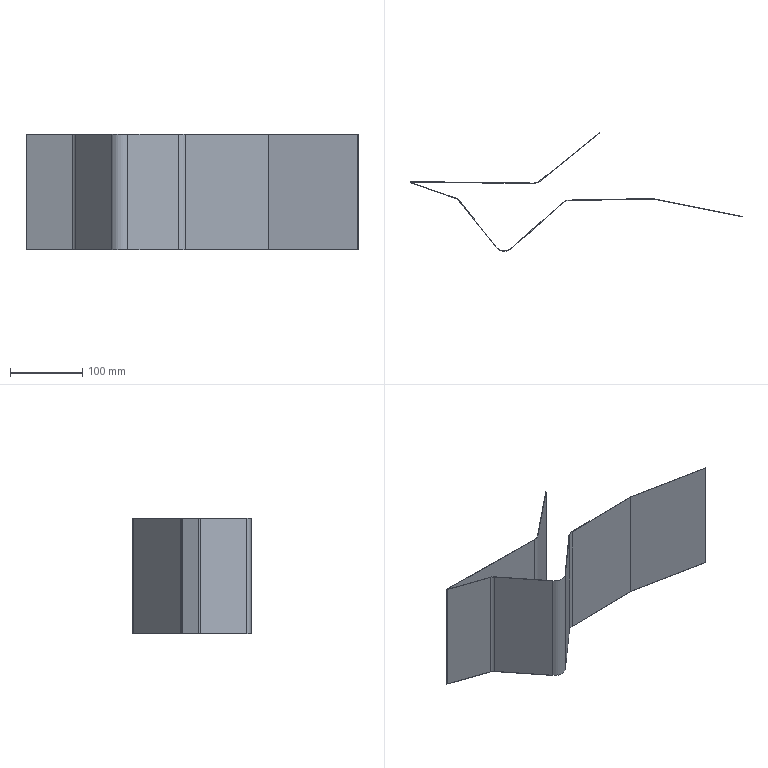Part | STEP file | Layout^ | 1 solid | 30 faces | box 459.008 x 163.495 x 160 mm | volume 64878 mm3 | plane 20 | cylinder 10 | commonest cylinder face diameters 30 x4 29 x2 31 x2 19 x1 20 x1
STEP:
#1=CARTESIAN_POINT('',(-164.589,156.602,25.));
#2=VERTEX_POINT('',#1);
#3=CARTESIAN_POINT('',(-41.59,132.165,25.));
#4=VERTEX_POINT('',#3);
#5=CARTESIAN_POINT('',(-164.642,156.612,25.));
#6=DIRECTION('',(0.9808,-0.1949,0.));
#7=VECTOR('',#6,1000.);
#8=LINE('',#5,#7);
#9=EDGE_CURVE('',#2,#4,#8,.T.);
#10=ORIENTED_EDGE('',*,*,#9,.T.);
#11=CARTESIAN_POINT('',(-41.59,132.165,185.));
#12=VERTEX_POINT('',#11);
#13=CARTESIAN_POINT('',(-41.59,132.165,185.));
#14=DIRECTION('',(0.,0.,-1.));
#15=VECTOR('',#14,1000.);
#16=LINE('',#13,#15);
#17=EDGE_CURVE('',#12,#4,#16,.T.);
#18=ORIENTED_EDGE('',*,*,#17,.F.);
#19=CARTESIAN_POINT('',(-164.589,156.602,185.));
#20=VERTEX_POINT('',#19);
#21=CARTESIAN_POINT('',(-164.642,156.612,185.));
#22=DIRECTION('',(0.9808,-0.1949,0.));
#23=VECTOR('',#22,1000.);
#24=LINE('',#21,#23);
#25=EDGE_CURVE('',#20,#12,#24,.T.);
#26=ORIENTED_EDGE('',*,*,#25,.F.);
#27=CARTESIAN_POINT('',(-164.589,156.602,185.));
#28=DIRECTION('',(0.,0.,-1.));
#29=VECTOR('',#28,1000.);
#30=LINE('',#27,#29);
#31=EDGE_CURVE('',#20,#2,#30,.T.);
#32=ORIENTED_EDGE('',*,*,#31,.T.);
#33=EDGE_LOOP('',(#10,#18,#26,#32));
#34=FACE_OUTER_BOUND('',#33,.T.);
#35=CARTESIAN_POINT('',(-164.642,156.612,185.));
#36=DIRECTION('',(0.1949,0.9808,0.));
#37=DIRECTION('',(-0.9808,0.1949,0.));
#38=AXIS2_PLACEMENT_3D('',#35,#36,#37);
#39=PLANE('',#38);
#40=ADVANCED_FACE('',(#34),#39,.F.);
#41=CARTESIAN_POINT('',(-41.492,132.655,25.));
#42=VERTEX_POINT('',#41);
#43=CARTESIAN_POINT('',(-41.492,132.655,25.));
#44=DIRECTION('',(-0.1949,-0.9808,0.));
#45=VECTOR('',#44,1000.);
#46=LINE('',#43,#45);
#47=EDGE_CURVE('',#42,#4,#46,.T.);
#48=ORIENTED_EDGE('',*,*,#47,.F.);
#49=CARTESIAN_POINT('',(-41.492,132.655,185.));
#50=VERTEX_POINT('',#49);
#51=CARTESIAN_POINT('',(-41.492,132.655,185.));
#52=DIRECTION('',(0.,0.,-1.));
#53=VECTOR('',#52,1000.);
#54=LINE('',#51,#53);
#55=EDGE_CURVE('',#50,#42,#54,.T.);
#56=ORIENTED_EDGE('',*,*,#55,.F.);
#57=CARTESIAN_POINT('',(-41.492,132.655,185.));
#58=DIRECTION('',(-0.1949,-0.9808,0.));
#59=VECTOR('',#58,1000.);
#60=LINE('',#57,#59);
#61=EDGE_CURVE('',#50,#12,#60,.T.);
#62=ORIENTED_EDGE('',*,*,#61,.T.);
#63=ORIENTED_EDGE('',*,*,#17,.T.);
#64=EDGE_LOOP('',(#48,#56,#62,#63));
#65=FACE_OUTER_BOUND('',#64,.T.);
#66=CARTESIAN_POINT('',(-41.492,132.655,185.));
#67=DIRECTION('',(0.9808,-0.1949,0.));
#68=DIRECTION('',(0.1949,0.9808,0.));
#69=AXIS2_PLACEMENT_3D('',#66,#67,#68);
#70=PLANE('',#69);
#71=ADVANCED_FACE('',(#65),#70,.T.);
#72=CARTESIAN_POINT('',(-164.544,157.103,25.));
#73=VERTEX_POINT('',#72);
#74=CARTESIAN_POINT('',(-164.544,157.103,25.));
#75=DIRECTION('',(0.9808,-0.1949,0.));
#76=VECTOR('',#75,1000.);
#77=LINE('',#74,#76);
#78=EDGE_CURVE('',#73,#42,#77,.T.);
#79=ORIENTED_EDGE('',*,*,#78,.F.);
#80=CARTESIAN_POINT('',(-164.544,157.103,185.));
#81=VERTEX_POINT('',#80);
#82=CARTESIAN_POINT('',(-164.544,157.103,185.));
#83=DIRECTION('',(0.,0.,-1.));
#84=VECTOR('',#83,1000.);
#85=LINE('',#82,#84);
#86=EDGE_CURVE('',#81,#73,#85,.T.);
#87=ORIENTED_EDGE('',*,*,#86,.F.);
#88=CARTESIAN_POINT('',(-164.544,157.103,185.));
#89=DIRECTION('',(0.9808,-0.1949,0.));
#90=VECTOR('',#89,1000.);
#91=LINE('',#88,#90);
#92=EDGE_CURVE('',#81,#50,#91,.T.);
#93=ORIENTED_EDGE('',*,*,#92,.T.);
#94=ORIENTED_EDGE('',*,*,#55,.T.);
#95=EDGE_LOOP('',(#79,#87,#93,#94));
#96=FACE_OUTER_BOUND('',#95,.T.);
#97=CARTESIAN_POINT('',(-164.544,157.103,185.));
#98=DIRECTION('',(0.1949,0.9808,0.));
#99=DIRECTION('',(-0.9808,0.1949,0.));
#100=AXIS2_PLACEMENT_3D('',#97,#98,#99);
#101=PLANE('',#100);
#102=ADVANCED_FACE('',(#96),#101,.T.);
#103=CARTESIAN_POINT('',(-280.273,154.998,25.));
#104=VERTEX_POINT('',#103);
#105=CARTESIAN_POINT('',(-280.273,154.998,25.));
#106=DIRECTION('',(0.9998,0.01819,0.));
#107=VECTOR('',#106,1000.);
#108=LINE('',#105,#107);
#109=EDGE_CURVE('',#104,#73,#108,.T.);
#110=ORIENTED_EDGE('',*,*,#109,.F.);
#111=CARTESIAN_POINT('',(-280.273,154.998,185.));
#112=VERTEX_POINT('',#111);
#113=CARTESIAN_POINT('',(-280.273,154.998,185.));
#114=DIRECTION('',(0.,0.,-1.));
#115=VECTOR('',#114,1000.);
#116=LINE('',#113,#115);
#117=EDGE_CURVE('',#112,#104,#116,.T.);
#118=ORIENTED_EDGE('',*,*,#117,.F.);
#119=CARTESIAN_POINT('',(-280.273,154.998,185.));
#120=DIRECTION('',(0.9998,0.01819,0.));
#121=VECTOR('',#120,1000.);
#122=LINE('',#119,#121);
#123=EDGE_CURVE('',#112,#81,#122,.T.);
#124=ORIENTED_EDGE('',*,*,#123,.T.);
#125=ORIENTED_EDGE('',*,*,#86,.T.);
#126=EDGE_LOOP('',(#110,#118,#124,#125));
#127=FACE_OUTER_BOUND('',#126,.T.);
#128=CARTESIAN_POINT('',(-280.273,154.998,185.));
#129=DIRECTION('',(-0.01819,0.9998,0.));
#130=DIRECTION('',(-0.9998,-0.01819,0.));
#131=AXIS2_PLACEMENT_3D('',#128,#129,#130);
#132=PLANE('',#131);
#133=ADVANCED_FACE('',(#127),#132,.T.);
#134=CARTESIAN_POINT('',(-289.978,151.2,25.));
#135=VERTEX_POINT('',#134);
#136=CARTESIAN_POINT('',(-280.,140.,25.));
#137=DIRECTION('',(0.,0.,-1.));
#138=DIRECTION('',(-1.,0.,0.));
#139=AXIS2_PLACEMENT_3D('',#136,#137,#138);
#140=CIRCLE('',#139,15.);
#141=EDGE_CURVE('',#135,#104,#140,.T.);
#142=ORIENTED_EDGE('',*,*,#141,.F.);
#143=CARTESIAN_POINT('',(-289.978,151.2,185.));
#144=VERTEX_POINT('',#143);
#145=CARTESIAN_POINT('',(-289.978,151.2,185.));
#146=DIRECTION('',(0.,0.,-1.));
#147=VECTOR('',#146,1000.);
#148=LINE('',#145,#147);
#149=EDGE_CURVE('',#144,#135,#148,.T.);
#150=ORIENTED_EDGE('',*,*,#149,.F.);
#151=CARTESIAN_POINT('',(-280.,140.,185.));
#152=DIRECTION('',(0.,0.,-1.));
#153=DIRECTION('',(-1.,0.,0.));
#154=AXIS2_PLACEMENT_3D('',#151,#152,#153);
#155=CIRCLE('',#154,15.);
#156=EDGE_CURVE('',#144,#112,#155,.T.);
#157=ORIENTED_EDGE('',*,*,#156,.T.);
#158=ORIENTED_EDGE('',*,*,#117,.T.);
#159=EDGE_LOOP('',(#142,#150,#157,#158));
#160=FACE_OUTER_BOUND('',#159,.T.);
#161=CARTESIAN_POINT('',(-280.,140.,185.));
#162=DIRECTION('',(0.,0.,-1.));
#163=DIRECTION('',(-1.,0.,0.));
#164=AXIS2_PLACEMENT_3D('',#161,#162,#163);
#165=CYLINDRICAL_SURFACE('',#164,15.);
#166=ADVANCED_FACE('',(#160),#165,.T.);
#167=CARTESIAN_POINT('',(-360.022,88.8,25.));
#168=VERTEX_POINT('',#167);
#169=CARTESIAN_POINT('',(-360.022,88.8,25.));
#170=DIRECTION('',(0.7467,0.6652,0.));
#171=VECTOR('',#170,1000.);
#172=LINE('',#169,#171);
#173=EDGE_CURVE('',#168,#135,#172,.T.);
#174=ORIENTED_EDGE('',*,*,#173,.F.);
#175=CARTESIAN_POINT('',(-360.022,88.8,185.));
#176=VERTEX_POINT('',#175);
#177=CARTESIAN_POINT('',(-360.022,88.8,185.));
#178=DIRECTION('',(0.,0.,-1.));
#179=VECTOR('',#178,1000.);
#180=LINE('',#177,#179);
#181=EDGE_CURVE('',#176,#168,#180,.T.);
#182=ORIENTED_EDGE('',*,*,#181,.F.);
#183=CARTESIAN_POINT('',(-360.022,88.8,185.));
#184=DIRECTION('',(0.7467,0.6652,0.));
#185=VECTOR('',#184,1000.);
#186=LINE('',#183,#185);
#187=EDGE_CURVE('',#176,#144,#186,.T.);
#188=ORIENTED_EDGE('',*,*,#187,.T.);
#189=ORIENTED_EDGE('',*,*,#149,.T.);
#190=EDGE_LOOP('',(#174,#182,#188,#189));
#191=FACE_OUTER_BOUND('',#190,.T.);
#192=CARTESIAN_POINT('',(-360.022,88.8,185.));
#193=DIRECTION('',(-0.6652,0.7467,0.));
#194=DIRECTION('',(-0.7467,-0.6652,0.));
#195=AXIS2_PLACEMENT_3D('',#192,#193,#194);
#196=PLANE('',#195);
#197=ADVANCED_FACE('',(#191),#196,.T.);
#198=CARTESIAN_POINT('',(-381.75,90.676,25.));
#199=VERTEX_POINT('',#198);
#200=CARTESIAN_POINT('',(-370.,100.,25.));
#201=DIRECTION('',(0.,0.,1.));
#202=DIRECTION('',(1.,0.,0.));
#203=AXIS2_PLACEMENT_3D('',#200,#201,#202);
#204=CIRCLE('',#203,15.);
#205=EDGE_CURVE('',#199,#168,#204,.T.);
#206=ORIENTED_EDGE('',*,*,#205,.F.);
#207=CARTESIAN_POINT('',(-381.75,90.676,185.));
#208=VERTEX_POINT('',#207);
#209=CARTESIAN_POINT('',(-381.75,90.676,185.));
#210=DIRECTION('',(0.,0.,-1.));
#211=VECTOR('',#210,1000.);
#212=LINE('',#209,#211);
#213=EDGE_CURVE('',#208,#199,#212,.T.);
#214=ORIENTED_EDGE('',*,*,#213,.F.);
#215=CARTESIAN_POINT('',(-370.,100.,185.));
#216=DIRECTION('',(0.,0.,1.));
#217=DIRECTION('',(1.,0.,0.));
#218=AXIS2_PLACEMENT_3D('',#215,#216,#217);
#219=CIRCLE('',#218,15.);
#220=EDGE_CURVE('',#208,#176,#219,.T.);
#221=ORIENTED_EDGE('',*,*,#220,.T.);
#222=ORIENTED_EDGE('',*,*,#181,.T.);
#223=EDGE_LOOP('',(#206,#214,#221,#222));
#224=FACE_OUTER_BOUND('',#223,.T.);
#225=CARTESIAN_POINT('',(-370.,100.,185.));
#226=DIRECTION('',(0.,0.,-1.));
#227=DIRECTION('',(-1.,0.,0.));
#228=AXIS2_PLACEMENT_3D('',#225,#226,#227);
#229=CYLINDRICAL_SURFACE('',#228,15.);
#230=ADVANCED_FACE('',(#224),#229,.F.);
#231=CARTESIAN_POINT('',(-432.166,154.216,25.));
#232=VERTEX_POINT('',#231);
#233=CARTESIAN_POINT('',(-432.166,154.216,25.));
#234=DIRECTION('',(0.6216,-0.7834,0.));
#235=VECTOR('',#234,1000.);
#236=LINE('',#233,#235);
#237=EDGE_CURVE('',#232,#199,#236,.T.);
#238=ORIENTED_EDGE('',*,*,#237,.F.);
#239=CARTESIAN_POINT('',(-432.166,154.216,185.));
#240=VERTEX_POINT('',#239);
#241=CARTESIAN_POINT('',(-432.166,154.216,185.));
#242=DIRECTION('',(0.,0.,-1.));
#243=VECTOR('',#242,1000.);
#244=LINE('',#241,#243);
#245=EDGE_CURVE('',#240,#232,#244,.T.);
#246=ORIENTED_EDGE('',*,*,#245,.F.);
#247=CARTESIAN_POINT('',(-432.166,154.216,185.));
#248=DIRECTION('',(0.6216,-0.7834,0.));
#249=VECTOR('',#248,1000.);
#250=LINE('',#247,#249);
#251=EDGE_CURVE('',#240,#208,#250,.T.);
#252=ORIENTED_EDGE('',*,*,#251,.T.);
#253=ORIENTED_EDGE('',*,*,#213,.T.);
#254=EDGE_LOOP('',(#238,#246,#252,#253));
#255=FACE_OUTER_BOUND('',#254,.T.);
#256=CARTESIAN_POINT('',(-432.166,154.216,185.));
#257=DIRECTION('',(0.7834,0.6216,0.));
#258=DIRECTION('',(-0.6216,0.7834,0.));
#259=AXIS2_PLACEMENT_3D('',#256,#257,#258);
#260=PLANE('',#259);
#261=ADVANCED_FACE('',(#255),#260,.T.);
#262=CARTESIAN_POINT('',(-436.696,157.438,25.));
#263=VERTEX_POINT('',#262);
#264=CARTESIAN_POINT('',(-440.,148.,25.));
#265=DIRECTION('',(0.,0.,-1.));
#266=DIRECTION('',(1.,0.,0.));
#267=AXIS2_PLACEMENT_3D('',#264,#265,#266);
#268=CIRCLE('',#267,10.);
#269=EDGE_CURVE('',#263,#232,#268,.T.);
#270=ORIENTED_EDGE('',*,*,#269,.F.);
#271=CARTESIAN_POINT('',(-436.696,157.438,185.));
#272=VERTEX_POINT('',#271);
#273=CARTESIAN_POINT('',(-436.696,157.438,185.));
#274=DIRECTION('',(0.,0.,-1.));
#275=VECTOR('',#274,1000.);
#276=LINE('',#273,#275);
#277=EDGE_CURVE('',#272,#263,#276,.T.);
#278=ORIENTED_EDGE('',*,*,#277,.F.);
#279=CARTESIAN_POINT('',(-440.,148.,185.));
#280=DIRECTION('',(0.,0.,-1.));
#281=DIRECTION('',(1.,0.,0.));
#282=AXIS2_PLACEMENT_3D('',#279,#280,#281);
#283=CIRCLE('',#282,10.);
#284=EDGE_CURVE('',#272,#240,#283,.T.);
#285=ORIENTED_EDGE('',*,*,#284,.T.);
#286=ORIENTED_EDGE('',*,*,#245,.T.);
#287=EDGE_LOOP('',(#270,#278,#285,#286));
#288=FACE_OUTER_BOUND('',#287,.T.);
#289=CARTESIAN_POINT('',(-440.,148.,185.));
#290=DIRECTION('',(0.,0.,-1.));
#291=DIRECTION('',(-1.,0.,0.));
#292=AXIS2_PLACEMENT_3D('',#289,#290,#291);
#293=CYLINDRICAL_SURFACE('',#292,10.);
#294=ADVANCED_FACE('',(#288),#293,.T.);
#295=CARTESIAN_POINT('',(-500.,179.6,25.));
#296=VERTEX_POINT('',#295);
#297=CARTESIAN_POINT('',(-500.,179.6,25.));
#298=DIRECTION('',(0.9438,-0.3304,0.));
#299=VECTOR('',#298,1000.);
#300=LINE('',#297,#299);
#301=EDGE_CURVE('',#296,#263,#300,.T.);
#302=ORIENTED_EDGE('',*,*,#301,.F.);
#303=CARTESIAN_POINT('',(-500.,179.6,185.));
#304=VERTEX_POINT('',#303);
#305=CARTESIAN_POINT('',(-500.,179.6,185.));
#306=DIRECTION('',(0.,0.,-1.));
#307=VECTOR('',#306,1000.);
#308=LINE('',#305,#307);
#309=EDGE_CURVE('',#304,#296,#308,.T.);
#310=ORIENTED_EDGE('',*,*,#309,.F.);
#311=CARTESIAN_POINT('',(-500.,179.6,185.));
#312=DIRECTION('',(0.9438,-0.3304,0.));
#313=VECTOR('',#312,1000.);
#314=LINE('',#311,#313);
#315=EDGE_CURVE('',#304,#272,#314,.T.);
#316=ORIENTED_EDGE('',*,*,#315,.T.);
#317=ORIENTED_EDGE('',*,*,#277,.T.);
#318=EDGE_LOOP('',(#302,#310,#316,#317));
#319=FACE_OUTER_BOUND('',#318,.T.);
#320=CARTESIAN_POINT('',(-500.,179.6,185.));
#321=DIRECTION('',(0.3304,0.9438,0.));
#322=DIRECTION('',(-0.9438,0.3304,0.));
#323=AXIS2_PLACEMENT_3D('',#320,#321,#322);
#324=PLANE('',#323);
#325=ADVANCED_FACE('',(#319),#324,.T.);
#326=CARTESIAN_POINT('',(-500.,180.,25.));
#327=VERTEX_POINT('',#326);
#328=CARTESIAN_POINT('',(-500.,180.,25.));
#329=DIRECTION('',(0.,-1.,0.));
#330=VECTOR('',#329,1000.);
#331=LINE('',#328,#330);
#332=EDGE_CURVE('',#327,#296,#331,.T.);
#333=ORIENTED_EDGE('',*,*,#332,.F.);
#334=CARTESIAN_POINT('',(-500.,180.,185.));
#335=VERTEX_POINT('',#334);
#336=CARTESIAN_POINT('',(-500.,180.,185.));
#337=DIRECTION('',(0.,0.,-1.));
#338=VECTOR('',#337,1000.);
#339=LINE('',#336,#338);
#340=EDGE_CURVE('',#335,#327,#339,.T.);
#341=ORIENTED_EDGE('',*,*,#340,.F.);
#342=CARTESIAN_POINT('',(-500.,180.,185.));
#343=DIRECTION('',(0.,-1.,0.));
#344=VECTOR('',#343,1000.);
#345=LINE('',#342,#344);
#346=EDGE_CURVE('',#335,#304,#345,.T.);
#347=ORIENTED_EDGE('',*,*,#346,.T.);
#348=ORIENTED_EDGE('',*,*,#309,.T.);
#349=EDGE_LOOP('',(#333,#341,#347,#348));
#350=FACE_OUTER_BOUND('',#349,.T.);
#351=CARTESIAN_POINT('',(-500.,180.,185.));
#352=DIRECTION('',(1.,0.,0.));
#353=DIRECTION('',(0.,0.,-1.));
#354=AXIS2_PLACEMENT_3D('',#351,#352,#353);
#355=PLANE('',#354);
#356=ADVANCED_FACE('',(#350),#355,.T.);
#357=CARTESIAN_POINT('',(-330.177,178.001,25.));
#358=VERTEX_POINT('',#357);
#359=CARTESIAN_POINT('',(-330.177,178.001,25.));
#360=DIRECTION('',(-0.9999,0.01177,0.));
#361=VECTOR('',#360,1000.);
#362=LINE('',#359,#361);
#363=EDGE_CURVE('',#358,#327,#362,.T.);
#364=ORIENTED_EDGE('',*,*,#363,.F.);
#365=CARTESIAN_POINT('',(-330.177,178.001,185.));
#366=VERTEX_POINT('',#365);
#367=CARTESIAN_POINT('',(-330.177,178.001,185.));
#368=DIRECTION('',(0.,0.,-1.));
#369=VECTOR('',#368,1000.);
#370=LINE('',#367,#369);
#371=EDGE_CURVE('',#366,#358,#370,.T.);
#372=ORIENTED_EDGE('',*,*,#371,.F.);
#373=CARTESIAN_POINT('',(-330.177,178.001,185.));
#374=DIRECTION('',(-0.9999,0.01177,0.));
#375=VECTOR('',#374,1000.);
#376=LINE('',#373,#375);
#377=EDGE_CURVE('',#366,#335,#376,.T.);
#378=ORIENTED_EDGE('',*,*,#377,.T.);
#379=ORIENTED_EDGE('',*,*,#340,.T.);
#380=EDGE_LOOP('',(#364,#372,#378,#379));
#381=FACE_OUTER_BOUND('',#380,.T.);
#382=CARTESIAN_POINT('',(-330.177,178.001,185.));
#383=DIRECTION('',(-0.01177,-0.9999,0.));
#384=DIRECTION('',(0.9999,-0.01177,0.));
#385=AXIS2_PLACEMENT_3D('',#382,#383,#384);
#386=PLANE('',#385);
#387=ADVANCED_FACE('',(#381),#386,.T.);
#388=CARTESIAN_POINT('',(-320.593,181.316,25.));
#389=VERTEX_POINT('',#388);
#390=CARTESIAN_POINT('',(-330.,193.,25.));
#391=DIRECTION('',(0.,0.,-1.));
#392=DIRECTION('',(-1.,0.,0.));
#393=AXIS2_PLACEMENT_3D('',#390,#391,#392);
#394=CIRCLE('',#393,15.);
#395=EDGE_CURVE('',#389,#358,#394,.T.);
#396=ORIENTED_EDGE('',*,*,#395,.F.);
#397=CARTESIAN_POINT('',(-320.593,181.316,185.));
#398=VERTEX_POINT('',#397);
#399=CARTESIAN_POINT('',(-320.593,181.316,185.));
#400=DIRECTION('',(0.,0.,-1.));
#401=VECTOR('',#400,1000.);
#402=LINE('',#399,#401);
#403=EDGE_CURVE('',#398,#389,#402,.T.);
#404=ORIENTED_EDGE('',*,*,#403,.F.);
#405=CARTESIAN_POINT('',(-330.,193.,185.));
#406=DIRECTION('',(0.,0.,-1.));
#407=DIRECTION('',(-1.,0.,0.));
#408=AXIS2_PLACEMENT_3D('',#405,#406,#407);
#409=CIRCLE('',#408,15.);
#410=EDGE_CURVE('',#398,#366,#409,.T.);
#411=ORIENTED_EDGE('',*,*,#410,.T.);
#412=ORIENTED_EDGE('',*,*,#371,.T.);
#413=EDGE_LOOP('',(#396,#404,#411,#412));
#414=FACE_OUTER_BOUND('',#413,.T.);
#415=CARTESIAN_POINT('',(-330.,193.,185.));
#416=DIRECTION('',(0.,0.,-1.));
#417=DIRECTION('',(-1.,0.,0.));
#418=AXIS2_PLACEMENT_3D('',#415,#416,#417);
#419=CYLINDRICAL_SURFACE('',#418,15.);
#420=ADVANCED_FACE('',(#414),#419,.T.);
#421=CARTESIAN_POINT('',(-239.407,246.684,25.));
#422=VERTEX_POINT('',#421);
#423=CARTESIAN_POINT('',(-239.407,246.684,25.));
#424=DIRECTION('',(-0.7789,-0.6271,0.));
#425=VECTOR('',#424,1000.);
#426=LINE('',#423,#425);
#427=EDGE_CURVE('',#422,#389,#426,.T.);
#428=ORIENTED_EDGE('',*,*,#427,.F.);
#429=CARTESIAN_POINT('',(-239.407,246.684,185.));
#430=VERTEX_POINT('',#429);
#431=CARTESIAN_POINT('',(-239.407,246.684,185.));
#432=DIRECTION('',(0.,0.,-1.));
#433=VECTOR('',#432,1000.);
#434=LINE('',#431,#433);
#435=EDGE_CURVE('',#430,#422,#434,.T.);
#436=ORIENTED_EDGE('',*,*,#435,.F.);
#437=CARTESIAN_POINT('',(-239.407,246.684,185.));
#438=DIRECTION('',(-0.7789,-0.6271,0.));
#439=VECTOR('',#438,1000.);
#440=LINE('',#437,#439);
#441=EDGE_CURVE('',#430,#398,#440,.T.);
#442=ORIENTED_EDGE('',*,*,#441,.T.);
#443=ORIENTED_EDGE('',*,*,#403,.T.);
#444=EDGE_LOOP('',(#428,#436,#442,#443));
#445=FACE_OUTER_BOUND('',#444,.T.);
#446=CARTESIAN_POINT('',(-239.407,246.684,185.));
#447=DIRECTION('',(0.6271,-0.7789,0.));
#448=DIRECTION('',(0.7789,0.6271,0.));
#449=AXIS2_PLACEMENT_3D('',#446,#447,#448);
#450=PLANE('',#449);
#451=ADVANCED_FACE('',(#445),#450,.T.);
#452=CARTESIAN_POINT('',(-238.176,247.576,25.));
#453=VERTEX_POINT('',#452);
#454=CARTESIAN_POINT('',(-230.,235.,25.));
#455=DIRECTION('',(0.,0.,1.));
#456=DIRECTION('',(-1.,0.,0.));
#457=AXIS2_PLACEMENT_3D('',#454,#455,#456);
#458=CIRCLE('',#457,15.);
#459=EDGE_CURVE('',#453,#422,#458,.T.);
#460=ORIENTED_EDGE('',*,*,#459,.F.);
#461=CARTESIAN_POINT('',(-238.176,247.576,185.));
#462=VERTEX_POINT('',#461);
#463=CARTESIAN_POINT('',(-238.176,247.576,185.));
#464=DIRECTION('',(0.,0.,-1.));
#465=VECTOR('',#464,1000.);
#466=LINE('',#463,#465);
#467=EDGE_CURVE('',#462,#453,#466,.T.);
#468=ORIENTED_EDGE('',*,*,#467,.F.);
#469=CARTESIAN_POINT('',(-230.,235.,185.));
#470=DIRECTION('',(0.,0.,1.));
#471=DIRECTION('',(-1.,0.,0.));
#472=AXIS2_PLACEMENT_3D('',#469,#470,#471);
#473=CIRCLE('',#472,15.);
#474=EDGE_CURVE('',#462,#430,#473,.T.);
#475=ORIENTED_EDGE('',*,*,#474,.T.);
#476=ORIENTED_EDGE('',*,*,#435,.T.);
#477=EDGE_LOOP('',(#460,#468,#475,#476));
#478=FACE_OUTER_BOUND('',#477,.T.);
#479=CARTESIAN_POINT('',(-230.,235.,185.));
#480=DIRECTION('',(0.,0.,-1.));
#481=DIRECTION('',(-1.,0.,0.));
#482=AXIS2_PLACEMENT_3D('',#479,#480,#481);
#483=CYLINDRICAL_SURFACE('',#482,15.);
#484=ADVANCED_FACE('',(#478),#483,.F.);
#485=CARTESIAN_POINT('',(-238.448,247.995,25.));
#486=VERTEX_POINT('',#485);
#487=CARTESIAN_POINT('',(-238.448,247.995,25.));
#488=DIRECTION('',(0.545,-0.8384,0.));
#489=VECTOR('',#488,1000.);
#490=LINE('',#487,#489);
#491=EDGE_CURVE('',#486,#453,#490,.T.);
#492=ORIENTED_EDGE('',*,*,#491,.F.);
#493=CARTESIAN_POINT('',(-238.448,247.995,185.));
#494=VERTEX_POINT('',#493);
#495=CARTESIAN_POINT('',(-238.448,247.995,185.));
#496=DIRECTION('',(0.,0.,-1.));
#497=VECTOR('',#496,1000.);
#498=LINE('',#495,#497);
#499=EDGE_CURVE('',#494,#486,#498,.T.);
#500=ORIENTED_EDGE('',*,*,#499,.F.);
#501=CARTESIAN_POINT('',(-238.448,247.995,185.));
#502=DIRECTION('',(0.545,-0.8384,0.));
#503=VECTOR('',#502,1000.);
#504=LINE('',#501,#503);
#505=EDGE_CURVE('',#494,#462,#504,.T.);
#506=ORIENTED_EDGE('',*,*,#505,.T.);
#507=ORIENTED_EDGE('',*,*,#467,.T.);
#508=EDGE_LOOP('',(#492,#500,#506,#507));
#509=FACE_OUTER_BOUND('',#508,.T.);
#510=CARTESIAN_POINT('',(-238.448,247.995,185.));
#511=DIRECTION('',(0.8384,0.545,0.));
#512=DIRECTION('',(-0.545,0.8384,0.));
#513=AXIS2_PLACEMENT_3D('',#510,#511,#512);
#514=PLANE('',#513);
#515=ADVANCED_FACE('',(#509),#514,.T.);
#516=CARTESIAN_POINT('',(-239.721,247.073,25.));
#517=VERTEX_POINT('',#516);
#518=CARTESIAN_POINT('',(-230.,235.,25.));
#519=DIRECTION('',(0.,0.,1.));
#520=DIRECTION('',(1.,0.,0.));
#521=AXIS2_PLACEMENT_3D('',#518,#519,#520);
#522=CIRCLE('',#521,15.5);
#523=EDGE_CURVE('',#486,#517,#522,.T.);
#524=ORIENTED_EDGE('',*,*,#523,.T.);
#525=CARTESIAN_POINT('',(-239.721,247.073,185.));
#526=VERTEX_POINT('',#525);
#527=CARTESIAN_POINT('',(-239.721,247.073,185.));
#528=DIRECTION('',(0.,0.,-1.));
#529=VECTOR('',#528,1000.);
#530=LINE('',#527,#529);
#531=EDGE_CURVE('',#526,#517,#530,.T.);
#532=ORIENTED_EDGE('',*,*,#531,.F.);
#533=CARTESIAN_POINT('',(-230.,235.,185.));
#534=DIRECTION('',(0.,0.,1.));
#535=DIRECTION('',(1.,0.,0.));
#536=AXIS2_PLACEMENT_3D('',#533,#534,#535);
#537=CIRCLE('',#536,15.5);
#538=EDGE_CURVE('',#494,#526,#537,.T.);
#539=ORIENTED_EDGE('',*,*,#538,.F.);
#540=ORIENTED_EDGE('',*,*,#499,.T.);
#541=EDGE_LOOP('',(#524,#532,#539,#540));
#542=FACE_OUTER_BOUND('',#541,.T.);
#543=CARTESIAN_POINT('',(-230.,235.,185.));
#544=DIRECTION('',(0.,0.,-1.));
#545=DIRECTION('',(-1.,0.,0.));
#546=AXIS2_PLACEMENT_3D('',#543,#544,#545);
#547=CYLINDRICAL_SURFACE('',#546,15.5);
#548=ADVANCED_FACE('',(#542),#547,.T.);
#549=CARTESIAN_POINT('',(-320.906,181.706,25.));
#550=VERTEX_POINT('',#549);
#551=CARTESIAN_POINT('',(-239.721,247.073,25.));
#552=DIRECTION('',(-0.7789,-0.6271,0.));
#553=VECTOR('',#552,1000.);
#554=LINE('',#551,#553);
#555=EDGE_CURVE('',#517,#550,#554,.T.);
#556=ORIENTED_EDGE('',*,*,#555,.T.);
#557=CARTESIAN_POINT('',(-320.906,181.706,185.));
#558=VERTEX_POINT('',#557);
#559=CARTESIAN_POINT('',(-320.906,181.706,185.));
#560=DIRECTION('',(0.,0.,-1.));
#561=VECTOR('',#560,1000.);
#562=LINE('',#559,#561);
#563=EDGE_CURVE('',#558,#550,#562,.T.);
#564=ORIENTED_EDGE('',*,*,#563,.F.);
#565=CARTESIAN_POINT('',(-239.721,247.073,185.));
#566=DIRECTION('',(-0.7789,-0.6271,0.));
#567=VECTOR('',#566,1000.);
#568=LINE('',#565,#567);
#569=EDGE_CURVE('',#526,#558,#568,.T.);
#570=ORIENTED_EDGE('',*,*,#569,.F.);
#571=ORIENTED_EDGE('',*,*,#531,.T.);
#572=EDGE_LOOP('',(#556,#564,#570,#571));
#573=FACE_OUTER_BOUND('',#572,.T.);
#574=CARTESIAN_POINT('',(-239.721,247.073,185.));
#575=DIRECTION('',(0.6271,-0.7789,0.));
#576=DIRECTION('',(0.7789,0.6271,0.));
#577=AXIS2_PLACEMENT_3D('',#574,#575,#576);
#578=PLANE('',#577);
#579=ADVANCED_FACE('',(#573),#578,.F.);
#580=CARTESIAN_POINT('',(-330.171,178.501,25.));
#581=VERTEX_POINT('',#580);
#582=CARTESIAN_POINT('',(-330.,193.,25.));
#583=DIRECTION('',(0.,0.,-1.));
#584=DIRECTION('',(1.,0.,0.));
#585=AXIS2_PLACEMENT_3D('',#582,#583,#584);
#586=CIRCLE('',#585,14.5);
#587=EDGE_CURVE('',#550,#581,#586,.T.);
#588=ORIENTED_EDGE('',*,*,#587,.T.);
#589=CARTESIAN_POINT('',(-330.171,178.501,185.));
#590=VERTEX_POINT('',#589);
#591=CARTESIAN_POINT('',(-330.171,178.501,185.));
#592=DIRECTION('',(0.,0.,-1.));
#593=VECTOR('',#592,1000.);
#594=LINE('',#591,#593);
#595=EDGE_CURVE('',#590,#581,#594,.T.);
#596=ORIENTED_EDGE('',*,*,#595,.F.);
#597=CARTESIAN_POINT('',(-330.,193.,185.));
#598=DIRECTION('',(0.,0.,-1.));
#599=DIRECTION('',(1.,0.,0.));
#600=AXIS2_PLACEMENT_3D('',#597,#598,#599);
#601=CIRCLE('',#600,14.5);
#602=EDGE_CURVE('',#558,#590,#601,.T.);
#603=ORIENTED_EDGE('',*,*,#602,.F.);
#604=ORIENTED_EDGE('',*,*,#563,.T.);
#605=EDGE_LOOP('',(#588,#596,#603,#604));
#606=FACE_OUTER_BOUND('',#605,.T.);
#607=CARTESIAN_POINT('',(-330.,193.,185.));
#608=DIRECTION('',(0.,0.,-1.));
#609=DIRECTION('',(-1.,0.,0.));
#610=AXIS2_PLACEMENT_3D('',#607,#608,#609);
#611=CYLINDRICAL_SURFACE('',#610,14.5);
#612=ADVANCED_FACE('',(#606),#611,.F.);
#613=CARTESIAN_POINT('',(-500.5,180.506,25.));
#614=VERTEX_POINT('',#613);
#615=CARTESIAN_POINT('',(-330.171,178.501,25.));
#616=DIRECTION('',(-0.9999,0.01177,0.));
#617=VECTOR('',#616,1000.);
#618=LINE('',#615,#617);
#619=EDGE_CURVE('',#581,#614,#618,.T.);
#620=ORIENTED_EDGE('',*,*,#619,.T.);
#621=CARTESIAN_POINT('',(-500.5,180.506,185.));
#622=VERTEX_POINT('',#621);
#623=CARTESIAN_POINT('',(-500.5,180.506,185.));
#624=DIRECTION('',(0.,0.,-1.));
#625=VECTOR('',#624,1000.);
#626=LINE('',#623,#625);
#627=EDGE_CURVE('',#622,#614,#626,.T.);
#628=ORIENTED_EDGE('',*,*,#627,.F.);
#629=CARTESIAN_POINT('',(-330.171,178.501,185.));
#630=DIRECTION('',(-0.9999,0.01177,0.));
#631=VECTOR('',#630,1000.);
#632=LINE('',#629,#631);
#633=EDGE_CURVE('',#590,#622,#632,.T.);
#634=ORIENTED_EDGE('',*,*,#633,.F.);
#635=ORIENTED_EDGE('',*,*,#595,.T.);
#636=EDGE_LOOP('',(#620,#628,#634,#635));
#637=FACE_OUTER_BOUND('',#636,.T.);
#638=CARTESIAN_POINT('',(-330.171,178.501,185.));
#639=DIRECTION('',(-0.01177,-0.9999,0.));
#640=DIRECTION('',(0.9999,-0.01177,0.));
#641=AXIS2_PLACEMENT_3D('',#638,#639,#640);
#642=PLANE('',#641);
#643=ADVANCED_FACE('',(#637),#642,.F.);
#644=CARTESIAN_POINT('',(-500.5,179.245,25.));
#645=VERTEX_POINT('',#644);
#646=CARTESIAN_POINT('',(-500.5,180.,25.));
#647=DIRECTION('',(0.,-1.,0.));
#648=VECTOR('',#647,1000.);
#649=LINE('',#646,#648);
#650=EDGE_CURVE('',#614,#645,#649,.T.);
#651=ORIENTED_EDGE('',*,*,#650,.T.);
#652=CARTESIAN_POINT('',(-500.5,179.245,185.));
#653=VERTEX_POINT('',#652);
#654=CARTESIAN_POINT('',(-500.5,179.245,185.));
#655=DIRECTION('',(0.,0.,-1.));
#656=VECTOR('',#655,1000.);
#657=LINE('',#654,#656);
#658=EDGE_CURVE('',#653,#645,#657,.T.);
#659=ORIENTED_EDGE('',*,*,#658,.F.);
#660=CARTESIAN_POINT('',(-500.5,180.,185.));
#661=DIRECTION('',(0.,-1.,0.));
#662=VECTOR('',#661,1000.);
#663=LINE('',#660,#662);
#664=EDGE_CURVE('',#622,#653,#663,.T.);
#665=ORIENTED_EDGE('',*,*,#664,.F.);
#666=ORIENTED_EDGE('',*,*,#627,.T.);
#667=EDGE_LOOP('',(#651,#659,#665,#666));
#668=FACE_OUTER_BOUND('',#667,.T.);
#669=CARTESIAN_POINT('',(-500.5,180.,185.));
#670=DIRECTION('',(1.,0.,0.));
#671=DIRECTION('',(0.,0.,-1.));
#672=AXIS2_PLACEMENT_3D('',#669,#670,#671);
#673=PLANE('',#672);
#674=ADVANCED_FACE('',(#668),#673,.F.);
#675=CARTESIAN_POINT('',(-436.861,156.966,25.));
#676=VERTEX_POINT('',#675);
#677=CARTESIAN_POINT('',(-500.165,179.128,25.));
#678=DIRECTION('',(0.9438,-0.3304,0.));
#679=VECTOR('',#678,1000.);
#680=LINE('',#677,#679);
#681=EDGE_CURVE('',#645,#676,#680,.T.);
#682=ORIENTED_EDGE('',*,*,#681,.T.);
#683=CARTESIAN_POINT('',(-436.861,156.966,185.));
#684=VERTEX_POINT('',#683);
#685=CARTESIAN_POINT('',(-436.861,156.966,185.));
#686=DIRECTION('',(0.,0.,-1.));
#687=VECTOR('',#686,1000.);
#688=LINE('',#685,#687);
#689=EDGE_CURVE('',#684,#676,#688,.T.);
#690=ORIENTED_EDGE('',*,*,#689,.F.);
#691=CARTESIAN_POINT('',(-500.165,179.128,185.));
#692=DIRECTION('',(0.9438,-0.3304,0.));
#693=VECTOR('',#692,1000.);
#694=LINE('',#691,#693);
#695=EDGE_CURVE('',#653,#684,#694,.T.);
#696=ORIENTED_EDGE('',*,*,#695,.F.);
#697=ORIENTED_EDGE('',*,*,#658,.T.);
#698=EDGE_LOOP('',(#682,#690,#696,#697));
#699=FACE_OUTER_BOUND('',#698,.T.);
#700=CARTESIAN_POINT('',(-500.165,179.128,185.));
#701=DIRECTION('',(0.3304,0.9438,0.));
#702=DIRECTION('',(-0.9438,0.3304,0.));
#703=AXIS2_PLACEMENT_3D('',#700,#701,#702);
#704=PLANE('',#703);
#705=ADVANCED_FACE('',(#699),#704,.F.);
#706=CARTESIAN_POINT('',(-432.558,153.905,25.));
#707=VERTEX_POINT('',#706);
#708=CARTESIAN_POINT('',(-440.,148.,25.));
#709=DIRECTION('',(0.,0.,-1.));
#710=DIRECTION('',(1.,0.,0.));
#711=AXIS2_PLACEMENT_3D('',#708,#709,#710);
#712=CIRCLE('',#711,9.5);
#713=EDGE_CURVE('',#676,#707,#712,.T.);
#714=ORIENTED_EDGE('',*,*,#713,.T.);
#715=CARTESIAN_POINT('',(-432.558,153.905,185.));
#716=VERTEX_POINT('',#715);
#717=CARTESIAN_POINT('',(-432.558,153.905,185.));
#718=DIRECTION('',(0.,0.,-1.));
#719=VECTOR('',#718,1000.);
#720=LINE('',#717,#719);
#721=EDGE_CURVE('',#716,#707,#720,.T.);
#722=ORIENTED_EDGE('',*,*,#721,.F.);
#723=CARTESIAN_POINT('',(-440.,148.,185.));
#724=DIRECTION('',(0.,0.,-1.));
#725=DIRECTION('',(1.,0.,0.));
#726=AXIS2_PLACEMENT_3D('',#723,#724,#725);
#727=CIRCLE('',#726,9.5);
#728=EDGE_CURVE('',#684,#716,#727,.T.);
#729=ORIENTED_EDGE('',*,*,#728,.F.);
#730=ORIENTED_EDGE('',*,*,#689,.T.);
#731=EDGE_LOOP('',(#714,#722,#729,#730));
#732=FACE_OUTER_BOUND('',#731,.T.);
#733=CARTESIAN_POINT('',(-440.,148.,185.));
#734=DIRECTION('',(0.,0.,-1.));
#735=DIRECTION('',(-1.,0.,0.));
#736=AXIS2_PLACEMENT_3D('',#733,#734,#735);
#737=CYLINDRICAL_SURFACE('',#736,9.5);
#738=ADVANCED_FACE('',(#732),#737,.F.);
#739=CARTESIAN_POINT('',(-382.142,90.366,25.));
#740=VERTEX_POINT('',#739);
#741=CARTESIAN_POINT('',(-432.558,153.905,25.));
#742=DIRECTION('',(0.6216,-0.7834,0.));
#743=VECTOR('',#742,1000.);
#744=LINE('',#741,#743);
#745=EDGE_CURVE('',#707,#740,#744,.T.);
#746=ORIENTED_EDGE('',*,*,#745,.T.);
#747=CARTESIAN_POINT('',(-382.142,90.366,185.));
#748=VERTEX_POINT('',#747);
#749=CARTESIAN_POINT('',(-382.142,90.366,185.));
#750=DIRECTION('',(0.,0.,-1.));
#751=VECTOR('',#750,1000.);
#752=LINE('',#749,#751);
#753=EDGE_CURVE('',#748,#740,#752,.T.);
#754=ORIENTED_EDGE('',*,*,#753,.F.);
#755=CARTESIAN_POINT('',(-432.558,153.905,185.));
#756=DIRECTION('',(0.6216,-0.7834,0.));
#757=VECTOR('',#756,1000.);
#758=LINE('',#755,#757);
#759=EDGE_CURVE('',#716,#748,#758,.T.);
#760=ORIENTED_EDGE('',*,*,#759,.F.);
#761=ORIENTED_EDGE('',*,*,#721,.T.);
#762=EDGE_LOOP('',(#746,#754,#760,#761));
#763=FACE_OUTER_BOUND('',#762,.T.);
#764=CARTESIAN_POINT('',(-432.558,153.905,185.));
#765=DIRECTION('',(0.7834,0.6216,0.));
#766=DIRECTION('',(-0.6216,0.7834,0.));
#767=AXIS2_PLACEMENT_3D('',#764,#765,#766);
#768=PLANE('',#767);
#769=ADVANCED_FACE('',(#763),#768,.F.);
#770=CARTESIAN_POINT('',(-359.69,88.427,25.));
#771=VERTEX_POINT('',#770);
#772=CARTESIAN_POINT('',(-370.,100.,25.));
#773=DIRECTION('',(0.,0.,1.));
#774=DIRECTION('',(1.,0.,0.));
#775=AXIS2_PLACEMENT_3D('',#772,#773,#774);
#776=CIRCLE('',#775,15.5);
#777=EDGE_CURVE('',#740,#771,#776,.T.);
#778=ORIENTED_EDGE('',*,*,#777,.T.);
#779=CARTESIAN_POINT('',(-359.69,88.427,185.));
#780=VERTEX_POINT('',#779);
#781=CARTESIAN_POINT('',(-359.69,88.427,185.));
#782=DIRECTION('',(0.,0.,-1.));
#783=VECTOR('',#782,1000.);
#784=LINE('',#781,#783);
#785=EDGE_CURVE('',#780,#771,#784,.T.);
#786=ORIENTED_EDGE('',*,*,#785,.F.);
#787=CARTESIAN_POINT('',(-370.,100.,185.));
#788=DIRECTION('',(0.,0.,1.));
#789=DIRECTION('',(1.,0.,0.));
#790=AXIS2_PLACEMENT_3D('',#787,#788,#789);
#791=CIRCLE('',#790,15.5);
#792=EDGE_CURVE('',#748,#780,#791,.T.);
#793=ORIENTED_EDGE('',*,*,#792,.F.);
#794=ORIENTED_EDGE('',*,*,#753,.T.);
#795=EDGE_LOOP('',(#778,#786,#793,#794));
#796=FACE_OUTER_BOUND('',#795,.T.);
#797=CARTESIAN_POINT('',(-370.,100.,185.));
#798=DIRECTION('',(0.,0.,-1.));
#799=DIRECTION('',(-1.,0.,0.));
#800=AXIS2_PLACEMENT_3D('',#797,#798,#799);
#801=CYLINDRICAL_SURFACE('',#800,15.5);
#802=ADVANCED_FACE('',(#796),#801,.T.);
#803=CARTESIAN_POINT('',(-289.645,150.827,25.));
#804=VERTEX_POINT('',#803);
#805=CARTESIAN_POINT('',(-359.69,88.427,25.));
#806=DIRECTION('',(0.7467,0.6652,0.));
#807=VECTOR('',#806,1000.);
#808=LINE('',#805,#807);
#809=EDGE_CURVE('',#771,#804,#808,.T.);
#810=ORIENTED_EDGE('',*,*,#809,.T.);
#811=CARTESIAN_POINT('',(-289.645,150.827,185.));
#812=VERTEX_POINT('',#811);
#813=CARTESIAN_POINT('',(-289.645,150.827,185.));
#814=DIRECTION('',(0.,0.,-1.));
#815=VECTOR('',#814,1000.);
#816=LINE('',#813,#815);
#817=EDGE_CURVE('',#812,#804,#816,.T.);
#818=ORIENTED_EDGE('',*,*,#817,.F.);
#819=CARTESIAN_POINT('',(-359.69,88.427,185.));
#820=DIRECTION('',(0.7467,0.6652,0.));
#821=VECTOR('',#820,1000.);
#822=LINE('',#819,#821);
#823=EDGE_CURVE('',#780,#812,#822,.T.);
#824=ORIENTED_EDGE('',*,*,#823,.F.);
#825=ORIENTED_EDGE('',*,*,#785,.T.);
#826=EDGE_LOOP('',(#810,#818,#824,#825));
#827=FACE_OUTER_BOUND('',#826,.T.);
#828=CARTESIAN_POINT('',(-359.69,88.427,185.));
#829=DIRECTION('',(-0.6652,0.7467,0.));
#830=DIRECTION('',(-0.7467,-0.6652,0.));
#831=AXIS2_PLACEMENT_3D('',#828,#829,#830);
#832=PLANE('',#831);
#833=ADVANCED_FACE('',(#827),#832,.F.);
#834=CARTESIAN_POINT('',(-280.264,154.498,25.));
#835=VERTEX_POINT('',#834);
#836=CARTESIAN_POINT('',(-280.,140.,25.));
#837=DIRECTION('',(0.,0.,-1.));
#838=DIRECTION('',(1.,0.,0.));
#839=AXIS2_PLACEMENT_3D('',#836,#837,#838);
#840=CIRCLE('',#839,14.5);
#841=EDGE_CURVE('',#804,#835,#840,.T.);
#842=ORIENTED_EDGE('',*,*,#841,.T.);
#843=CARTESIAN_POINT('',(-280.264,154.498,185.));
#844=VERTEX_POINT('',#843);
#845=CARTESIAN_POINT('',(-280.264,154.498,185.));
#846=DIRECTION('',(0.,0.,-1.));
#847=VECTOR('',#846,1000.);
#848=LINE('',#845,#847);
#849=EDGE_CURVE('',#844,#835,#848,.T.);
#850=ORIENTED_EDGE('',*,*,#849,.F.);
#851=CARTESIAN_POINT('',(-280.,140.,185.));
#852=DIRECTION('',(0.,0.,-1.));
#853=DIRECTION('',(1.,0.,0.));
#854=AXIS2_PLACEMENT_3D('',#851,#852,#853);
#855=CIRCLE('',#854,14.5);
#856=EDGE_CURVE('',#812,#844,#855,.T.);
#857=ORIENTED_EDGE('',*,*,#856,.F.);
#858=ORIENTED_EDGE('',*,*,#817,.T.);
#859=EDGE_LOOP('',(#842,#850,#857,#858));
#860=FACE_OUTER_BOUND('',#859,.T.);
#861=CARTESIAN_POINT('',(-280.,140.,185.));
#862=DIRECTION('',(0.,0.,-1.));
#863=DIRECTION('',(-1.,0.,0.));
#864=AXIS2_PLACEMENT_3D('',#861,#862,#863);
#865=CYLINDRICAL_SURFACE('',#864,14.5);
#866=ADVANCED_FACE('',(#860),#865,.F.);
#867=CARTESIAN_POINT('',(-280.264,154.498,25.));
#868=DIRECTION('',(0.9998,0.01819,0.));
#869=VECTOR('',#868,1000.);
#870=LINE('',#867,#869);
#871=EDGE_CURVE('',#835,#2,#870,.T.);
#872=ORIENTED_EDGE('',*,*,#871,.T.);
#873=ORIENTED_EDGE('',*,*,#31,.F.);
#874=CARTESIAN_POINT('',(-280.264,154.498,185.));
#875=DIRECTION('',(0.9998,0.01819,0.));
#876=VECTOR('',#875,1000.);
#877=LINE('',#874,#876);
#878=EDGE_CURVE('',#844,#20,#877,.T.);
#879=ORIENTED_EDGE('',*,*,#878,.F.);
#880=ORIENTED_EDGE('',*,*,#849,.T.);
#881=EDGE_LOOP('',(#872,#873,#879,#880));
#882=FACE_OUTER_BOUND('',#881,.T.);
#883=CARTESIAN_POINT('',(-280.264,154.498,185.));
#884=DIRECTION('',(-0.01819,0.9998,0.));
#885=DIRECTION('',(-0.9998,-0.01819,0.));
#886=AXIS2_PLACEMENT_3D('',#883,#884,#885);
#887=PLANE('',#886);
#888=ADVANCED_FACE('',(#882),#887,.F.);
#889=ORIENTED_EDGE('',*,*,#25,.T.);
#890=ORIENTED_EDGE('',*,*,#61,.F.);
#891=ORIENTED_EDGE('',*,*,#92,.F.);
#892=ORIENTED_EDGE('',*,*,#123,.F.);
#893=ORIENTED_EDGE('',*,*,#156,.F.);
#894=ORIENTED_EDGE('',*,*,#187,.F.);
#895=ORIENTED_EDGE('',*,*,#220,.F.);
#896=ORIENTED_EDGE('',*,*,#251,.F.);
#897=ORIENTED_EDGE('',*,*,#284,.F.);
#898=ORIENTED_EDGE('',*,*,#315,.F.);
#899=ORIENTED_EDGE('',*,*,#346,.F.);
#900=ORIENTED_EDGE('',*,*,#377,.F.);
#901=ORIENTED_EDGE('',*,*,#410,.F.);
#902=ORIENTED_EDGE('',*,*,#441,.F.);
#903=ORIENTED_EDGE('',*,*,#474,.F.);
#904=ORIENTED_EDGE('',*,*,#505,.F.);
#905=ORIENTED_EDGE('',*,*,#538,.T.);
#906=ORIENTED_EDGE('',*,*,#569,.T.);
#907=ORIENTED_EDGE('',*,*,#602,.T.);
#908=ORIENTED_EDGE('',*,*,#633,.T.);
#909=ORIENTED_EDGE('',*,*,#664,.T.);
#910=ORIENTED_EDGE('',*,*,#695,.T.);
#911=ORIENTED_EDGE('',*,*,#728,.T.);
#912=ORIENTED_EDGE('',*,*,#759,.T.);
#913=ORIENTED_EDGE('',*,*,#792,.T.);
#914=ORIENTED_EDGE('',*,*,#823,.T.);
#915=ORIENTED_EDGE('',*,*,#856,.T.);
#916=ORIENTED_EDGE('',*,*,#878,.T.);
#917=EDGE_LOOP('',(#889,#890,#891,#892,#893,#894,#895,#896,#897,#898,#899,#900,#901,#902,#903,#904,#905,#906,#907,#908,#909,#910,#911,#912,#913,#914,#915,#916));
#918=FACE_OUTER_BOUND('',#917,.T.);
#919=CARTESIAN_POINT('',(-280.,140.,185.));
#920=DIRECTION('',(0.,0.,-1.));
#921=DIRECTION('',(-1.,0.,0.));
#922=AXIS2_PLACEMENT_3D('',#919,#920,#921);
#923=PLANE('',#922);
#924=ADVANCED_FACE('',(#918),#923,.F.);
#925=ORIENTED_EDGE('',*,*,#9,.F.);
#926=ORIENTED_EDGE('',*,*,#871,.F.);
#927=ORIENTED_EDGE('',*,*,#841,.F.);
#928=ORIENTED_EDGE('',*,*,#809,.F.);
#929=ORIENTED_EDGE('',*,*,#777,.F.);
#930=ORIENTED_EDGE('',*,*,#745,.F.);
#931=ORIENTED_EDGE('',*,*,#713,.F.);
#932=ORIENTED_EDGE('',*,*,#681,.F.);
#933=ORIENTED_EDGE('',*,*,#650,.F.);
#934=ORIENTED_EDGE('',*,*,#619,.F.);
#935=ORIENTED_EDGE('',*,*,#587,.F.);
#936=ORIENTED_EDGE('',*,*,#555,.F.);
#937=ORIENTED_EDGE('',*,*,#523,.F.);
#938=ORIENTED_EDGE('',*,*,#491,.T.);
#939=ORIENTED_EDGE('',*,*,#459,.T.);
#940=ORIENTED_EDGE('',*,*,#427,.T.);
#941=ORIENTED_EDGE('',*,*,#395,.T.);
#942=ORIENTED_EDGE('',*,*,#363,.T.);
#943=ORIENTED_EDGE('',*,*,#332,.T.);
#944=ORIENTED_EDGE('',*,*,#301,.T.);
#945=ORIENTED_EDGE('',*,*,#269,.T.);
#946=ORIENTED_EDGE('',*,*,#237,.T.);
#947=ORIENTED_EDGE('',*,*,#205,.T.);
#948=ORIENTED_EDGE('',*,*,#173,.T.);
#949=ORIENTED_EDGE('',*,*,#141,.T.);
#950=ORIENTED_EDGE('',*,*,#109,.T.);
#951=ORIENTED_EDGE('',*,*,#78,.T.);
#952=ORIENTED_EDGE('',*,*,#47,.T.);
#953=EDGE_LOOP('',(#925,#926,#927,#928,#929,#930,#931,#932,#933,#934,#935,#936,#937,#938,#939,#940,#941,#942,#943,#944,#945,#946,#947,#948,#949,#950,#951,#952));
#954=FACE_OUTER_BOUND('',#953,.T.);
#955=CARTESIAN_POINT('',(-280.,140.,25.));
#956=DIRECTION('',(0.,0.,-1.));
#957=DIRECTION('',(-1.,0.,0.));
#958=AXIS2_PLACEMENT_3D('',#955,#956,#957);
#959=PLANE('',#958);
#960=ADVANCED_FACE('',(#954),#959,.T.);
#961=CLOSED_SHELL('',(#40,#71,#102,#133,#166,#197,#230,#261,#294,#325,#356,#387,#420,#451,#484,#515,#548,#579,#612,#643,#674,#705,#738,#769,#802,#833,#866,#888,#924,#960));
#962=MANIFOLD_SOLID_BREP('',#961);
#963=CARTESIAN_POINT('',(0.,0.,0.));
#964=DIRECTION('',(0.,0.,1.));
#965=DIRECTION('',(1.,0.,0.));
#966=AXIS2_PLACEMENT_3D('',#963,#964,#965);
#967=(LENGTH_UNIT()NAMED_UNIT(*)SI_UNIT(.MILLI.,.METRE.));
#968=UNCERTAINTY_MEASURE_WITH_UNIT(LENGTH_MEASURE(0.00001),#967,'','');
#969=(NAMED_UNIT(*)PLANE_ANGLE_UNIT()SI_UNIT($,.RADIAN.));
#970=(NAMED_UNIT(*)SI_UNIT($,.STERADIAN.)SOLID_ANGLE_UNIT());
#971=(GEOMETRIC_REPRESENTATION_CONTEXT(3)GLOBAL_UNCERTAINTY_ASSIGNED_CONTEXT((#968))GLOBAL_UNIT_ASSIGNED_CONTEXT((#967,#969,#970))REPRESENTATION_CONTEXT('',''));
#972=ADVANCED_BREP_SHAPE_REPRESENTATION('',(#962,#966),#971);